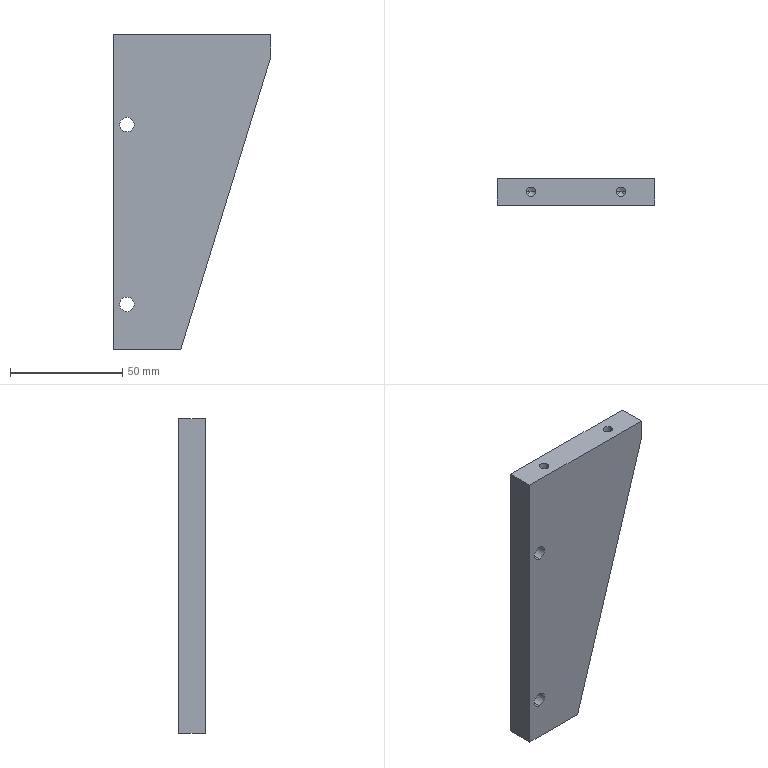Part | STEP file | PN_0033 | 1 solid | 19 faces | box 70 x 12 x 140 mm | volume 85204 mm3 | cylinder 8 | plane 7 | cone 4 | commonest cylinder face diameters 4.2 x4 6.5 x4
STEP:
#1=CARTESIAN_POINT('',(0.,0.,0.));
#2=DIRECTION('',(0.,0.,1.));
#3=DIRECTION('',(1.,0.,0.));
#4=AXIS2_PLACEMENT_3D('',#1,#2,#3);
#5=CARTESIAN_POINT('',(-17.9,6.,56.));
#6=VERTEX_POINT('',#5);
#7=CARTESIAN_POINT('',(-17.9,6.,70.));
#8=VERTEX_POINT('',#7);
#9=CARTESIAN_POINT('',(-17.9,6.,70.));
#10=DIRECTION('',(0.,0.,1.));
#11=VECTOR('',#10,1.);
#12=LINE('',#9,#11);
#13=CARTESIAN_POINT('',(-20.,6.,70.));
#14=DIRECTION('',(0.,0.,1.));
#15=DIRECTION('',(1.,0.,0.));
#16=AXIS2_PLACEMENT_3D('',#13,#14,#15);
#17=CYLINDRICAL_SURFACE('',#16,2.1);
#18=CARTESIAN_POINT('',(6.283,0.));
#19=DIRECTION('',(0.,1.));
#20=VECTOR('',#19,1.);
#21=LINE('',#18,#20);
#22=(GEOMETRIC_REPRESENTATION_CONTEXT(2)PARAMETRIC_REPRESENTATION_CONTEXT()REPRESENTATION_CONTEXT('',''));
#23=DEFINITIONAL_REPRESENTATION('',(#21),#22);
#24=PCURVE('',#17,#23);
#25=CARTESIAN_POINT('',(-20.,6.,70.));
#26=DIRECTION('',(0.,0.,1.));
#27=DIRECTION('',(1.,0.,0.));
#28=AXIS2_PLACEMENT_3D('',#25,#26,#27);
#29=CYLINDRICAL_SURFACE('',#28,2.1);
#30=CARTESIAN_POINT('',(0.,0.));
#31=DIRECTION('',(0.,1.));
#32=VECTOR('',#31,1.);
#33=LINE('',#30,#32);
#34=(GEOMETRIC_REPRESENTATION_CONTEXT(2)PARAMETRIC_REPRESENTATION_CONTEXT()REPRESENTATION_CONTEXT('',''));
#35=DEFINITIONAL_REPRESENTATION('',(#33),#34);
#36=PCURVE('',#29,#35);
#37=SURFACE_CURVE('',#12,(#24,#36),.PCURVE_S1.);
#38=EDGE_CURVE('',#6,#8,#37,.T.);
#39=ORIENTED_EDGE('',*,*,#38,.T.);
#40=CARTESIAN_POINT('',(-22.1,6.,70.));
#41=VERTEX_POINT('',#40);
#42=CARTESIAN_POINT('',(-20.,6.,70.));
#43=DIRECTION('',(0.,0.,1.));
#44=DIRECTION('',(1.,0.,0.));
#45=AXIS2_PLACEMENT_3D('',#42,#43,#44);
#46=CIRCLE('',#45,2.1);
#47=CARTESIAN_POINT('',(0.,0.));
#48=DIRECTION('',(1.,0.));
#49=VECTOR('',#48,1.);
#50=LINE('',#47,#49);
#51=(GEOMETRIC_REPRESENTATION_CONTEXT(2)PARAMETRIC_REPRESENTATION_CONTEXT()REPRESENTATION_CONTEXT('',''));
#52=DEFINITIONAL_REPRESENTATION('',(#50),#51);
#53=PCURVE('',#17,#52);
#54=CARTESIAN_POINT('',(-35.,12.,70.));
#55=DIRECTION('',(0.,0.,-1.));
#56=DIRECTION('',(-1.,0.,0.));
#57=AXIS2_PLACEMENT_3D('',#54,#55,#56);
#58=PLANE('',#57);
#59=CARTESIAN_POINT('',(-17.1,-6.));
#60=CARTESIAN_POINT('',(-17.1,-2.363));
#61=CARTESIAN_POINT('',(-13.95,-4.181));
#62=CARTESIAN_POINT('',(-10.8,-6.));
#63=CARTESIAN_POINT('',(-13.95,-7.819));
#64=CARTESIAN_POINT('',(-17.1,-9.637));
#65=CARTESIAN_POINT('',(-17.1,-6.));
#66=(BOUNDED_CURVE()B_SPLINE_CURVE(2,(#59,#60,#61,#62,#63,#64,#65),.UNSPECIFIED.,.T.,.F.)B_SPLINE_CURVE_WITH_KNOTS((1,2,2,2,2,1),(-2.094,0.,2.094,4.189,6.283,8.378),.UNSPECIFIED.)CURVE()GEOMETRIC_REPRESENTATION_ITEM()RATIONAL_B_SPLINE_CURVE((1.,0.5,1.,0.5,1.,0.5,1.))REPRESENTATION_ITEM(''));
#67=(GEOMETRIC_REPRESENTATION_CONTEXT(2)PARAMETRIC_REPRESENTATION_CONTEXT()REPRESENTATION_CONTEXT('',''));
#68=DEFINITIONAL_REPRESENTATION('',(#66),#67);
#69=PCURVE('',#58,#68);
#70=SURFACE_CURVE('',#46,(#53,#69),.PCURVE_S1.);
#71=EDGE_CURVE('',#41,#8,#70,.T.);
#72=ORIENTED_EDGE('',*,*,#71,.F.);
#73=CARTESIAN_POINT('',(-22.1,6.,56.));
#74=VERTEX_POINT('',#73);
#75=CARTESIAN_POINT('',(-22.1,6.,70.));
#76=DIRECTION('',(0.,0.,1.));
#77=VECTOR('',#76,1.);
#78=LINE('',#75,#77);
#79=CARTESIAN_POINT('',(3.142,0.));
#80=DIRECTION('',(0.,1.));
#81=VECTOR('',#80,1.);
#82=LINE('',#79,#81);
#83=(GEOMETRIC_REPRESENTATION_CONTEXT(2)PARAMETRIC_REPRESENTATION_CONTEXT()REPRESENTATION_CONTEXT('',''));
#84=DEFINITIONAL_REPRESENTATION('',(#82),#83);
#85=PCURVE('',#17,#84);
#86=CARTESIAN_POINT('',(3.142,0.));
#87=DIRECTION('',(0.,1.));
#88=VECTOR('',#87,1.);
#89=LINE('',#86,#88);
#90=(GEOMETRIC_REPRESENTATION_CONTEXT(2)PARAMETRIC_REPRESENTATION_CONTEXT()REPRESENTATION_CONTEXT('',''));
#91=DEFINITIONAL_REPRESENTATION('',(#89),#90);
#92=PCURVE('',#29,#91);
#93=SURFACE_CURVE('',#78,(#85,#92),.PCURVE_S1.);
#94=EDGE_CURVE('',#74,#41,#93,.T.);
#95=ORIENTED_EDGE('',*,*,#94,.F.);
#96=CARTESIAN_POINT('',(-20.,6.,56.));
#97=DIRECTION('',(0.,0.,1.));
#98=DIRECTION('',(1.,0.,0.));
#99=AXIS2_PLACEMENT_3D('',#96,#97,#98);
#100=CIRCLE('',#99,2.1);
#101=CARTESIAN_POINT('',(0.,-14.));
#102=DIRECTION('',(1.,0.));
#103=VECTOR('',#102,1.);
#104=LINE('',#101,#103);
#105=(GEOMETRIC_REPRESENTATION_CONTEXT(2)PARAMETRIC_REPRESENTATION_CONTEXT()REPRESENTATION_CONTEXT('',''));
#106=DEFINITIONAL_REPRESENTATION('',(#104),#105);
#107=PCURVE('',#17,#106);
#108=CARTESIAN_POINT('',(-20.,6.,56.));
#109=DIRECTION('',(0.,0.,1.));
#110=DIRECTION('',(1.,0.,0.));
#111=AXIS2_PLACEMENT_3D('',#108,#109,#110);
#112=CONICAL_SURFACE('',#111,2.1,1.03);
#113=CARTESIAN_POINT('',(0.,0.));
#114=DIRECTION('',(1.,0.));
#115=VECTOR('',#114,1.);
#116=LINE('',#113,#115);
#117=(GEOMETRIC_REPRESENTATION_CONTEXT(2)PARAMETRIC_REPRESENTATION_CONTEXT()REPRESENTATION_CONTEXT('',''));
#118=DEFINITIONAL_REPRESENTATION('',(#116),#117);
#119=PCURVE('',#112,#118);
#120=SURFACE_CURVE('',#100,(#107,#119),.PCURVE_S1.);
#121=EDGE_CURVE('',#74,#6,#120,.T.);
#122=ORIENTED_EDGE('',*,*,#121,.T.);
#123=EDGE_LOOP('',(#39,#72,#95,#122));
#124=FACE_BOUND('',#123,.F.);
#125=ADVANCED_FACE('',(#124),#17,.F.);
#126=ORIENTED_EDGE('',*,*,#121,.F.);
#127=CARTESIAN_POINT('',(-20.,6.,54.738));
#128=VERTEX_POINT('',#127);
#129=CARTESIAN_POINT('',(-22.1,6.,56.));
#130=DIRECTION('',(-0.8572,0.,0.515));
#131=VECTOR('',#130,1.);
#132=LINE('',#129,#131);
#133=CARTESIAN_POINT('',(3.142,0.));
#134=DIRECTION('',(0.,1.));
#135=VECTOR('',#134,1.);
#136=LINE('',#133,#135);
#137=(GEOMETRIC_REPRESENTATION_CONTEXT(2)PARAMETRIC_REPRESENTATION_CONTEXT()REPRESENTATION_CONTEXT('',''));
#138=DEFINITIONAL_REPRESENTATION('',(#136),#137);
#139=PCURVE('',#112,#138);
#140=CARTESIAN_POINT('',(-20.,6.,56.));
#141=DIRECTION('',(0.,0.,1.));
#142=DIRECTION('',(1.,0.,0.));
#143=AXIS2_PLACEMENT_3D('',#140,#141,#142);
#144=CONICAL_SURFACE('',#143,2.1,1.03);
#145=CARTESIAN_POINT('',(3.142,0.));
#146=DIRECTION('',(0.,1.));
#147=VECTOR('',#146,1.);
#148=LINE('',#145,#147);
#149=(GEOMETRIC_REPRESENTATION_CONTEXT(2)PARAMETRIC_REPRESENTATION_CONTEXT()REPRESENTATION_CONTEXT('',''));
#150=DEFINITIONAL_REPRESENTATION('',(#148),#149);
#151=PCURVE('',#144,#150);
#152=SURFACE_CURVE('',#132,(#139,#151),.PCURVE_S1.);
#153=EDGE_CURVE('',#128,#74,#152,.T.);
#154=ORIENTED_EDGE('',*,*,#153,.F.);
#155=CARTESIAN_POINT('',(-17.9,6.,56.));
#156=DIRECTION('',(0.8572,0.,0.515));
#157=VECTOR('',#156,1.);
#158=LINE('',#155,#157);
#159=CARTESIAN_POINT('',(6.283,0.));
#160=DIRECTION('',(0.,1.));
#161=VECTOR('',#160,1.);
#162=LINE('',#159,#161);
#163=(GEOMETRIC_REPRESENTATION_CONTEXT(2)PARAMETRIC_REPRESENTATION_CONTEXT()REPRESENTATION_CONTEXT('',''));
#164=DEFINITIONAL_REPRESENTATION('',(#162),#163);
#165=PCURVE('',#112,#164);
#166=CARTESIAN_POINT('',(0.,0.));
#167=DIRECTION('',(0.,1.));
#168=VECTOR('',#167,1.);
#169=LINE('',#166,#168);
#170=(GEOMETRIC_REPRESENTATION_CONTEXT(2)PARAMETRIC_REPRESENTATION_CONTEXT()REPRESENTATION_CONTEXT('',''));
#171=DEFINITIONAL_REPRESENTATION('',(#169),#170);
#172=PCURVE('',#144,#171);
#173=SURFACE_CURVE('',#158,(#165,#172),.PCURVE_S1.);
#174=EDGE_CURVE('',#128,#6,#173,.T.);
#175=ORIENTED_EDGE('',*,*,#174,.T.);
#176=EDGE_LOOP('',(#126,#154,#175));
#177=FACE_BOUND('',#176,.F.);
#178=ADVANCED_FACE('',(#177),#112,.F.);
#179=CARTESIAN_POINT('',(22.1,6.,56.));
#180=VERTEX_POINT('',#179);
#181=CARTESIAN_POINT('',(22.1,6.,70.));
#182=VERTEX_POINT('',#181);
#183=CARTESIAN_POINT('',(22.1,6.,70.));
#184=DIRECTION('',(0.,0.,1.));
#185=VECTOR('',#184,1.);
#186=LINE('',#183,#185);
#187=CARTESIAN_POINT('',(20.,6.,70.));
#188=DIRECTION('',(0.,0.,1.));
#189=DIRECTION('',(1.,0.,0.));
#190=AXIS2_PLACEMENT_3D('',#187,#188,#189);
#191=CYLINDRICAL_SURFACE('',#190,2.1);
#192=CARTESIAN_POINT('',(6.283,0.));
#193=DIRECTION('',(0.,1.));
#194=VECTOR('',#193,1.);
#195=LINE('',#192,#194);
#196=(GEOMETRIC_REPRESENTATION_CONTEXT(2)PARAMETRIC_REPRESENTATION_CONTEXT()REPRESENTATION_CONTEXT('',''));
#197=DEFINITIONAL_REPRESENTATION('',(#195),#196);
#198=PCURVE('',#191,#197);
#199=CARTESIAN_POINT('',(20.,6.,70.));
#200=DIRECTION('',(0.,0.,1.));
#201=DIRECTION('',(1.,0.,0.));
#202=AXIS2_PLACEMENT_3D('',#199,#200,#201);
#203=CYLINDRICAL_SURFACE('',#202,2.1);
#204=CARTESIAN_POINT('',(0.,0.));
#205=DIRECTION('',(0.,1.));
#206=VECTOR('',#205,1.);
#207=LINE('',#204,#206);
#208=(GEOMETRIC_REPRESENTATION_CONTEXT(2)PARAMETRIC_REPRESENTATION_CONTEXT()REPRESENTATION_CONTEXT('',''));
#209=DEFINITIONAL_REPRESENTATION('',(#207),#208);
#210=PCURVE('',#203,#209);
#211=SURFACE_CURVE('',#186,(#198,#210),.PCURVE_S1.);
#212=EDGE_CURVE('',#180,#182,#211,.T.);
#213=ORIENTED_EDGE('',*,*,#212,.T.);
#214=CARTESIAN_POINT('',(17.9,6.,70.));
#215=VERTEX_POINT('',#214);
#216=CARTESIAN_POINT('',(20.,6.,70.));
#217=DIRECTION('',(0.,0.,1.));
#218=DIRECTION('',(1.,0.,0.));
#219=AXIS2_PLACEMENT_3D('',#216,#217,#218);
#220=CIRCLE('',#219,2.1);
#221=CARTESIAN_POINT('',(0.,0.));
#222=DIRECTION('',(1.,0.));
#223=VECTOR('',#222,1.);
#224=LINE('',#221,#223);
#225=(GEOMETRIC_REPRESENTATION_CONTEXT(2)PARAMETRIC_REPRESENTATION_CONTEXT()REPRESENTATION_CONTEXT('',''));
#226=DEFINITIONAL_REPRESENTATION('',(#224),#225);
#227=PCURVE('',#191,#226);
#228=CARTESIAN_POINT('',(-57.1,-6.));
#229=CARTESIAN_POINT('',(-57.1,-2.363));
#230=CARTESIAN_POINT('',(-53.95,-4.181));
#231=CARTESIAN_POINT('',(-50.8,-6.));
#232=CARTESIAN_POINT('',(-53.95,-7.819));
#233=CARTESIAN_POINT('',(-57.1,-9.637));
#234=CARTESIAN_POINT('',(-57.1,-6.));
#235=(BOUNDED_CURVE()B_SPLINE_CURVE(2,(#228,#229,#230,#231,#232,#233,#234),.UNSPECIFIED.,.T.,.F.)B_SPLINE_CURVE_WITH_KNOTS((1,2,2,2,2,1),(-2.094,0.,2.094,4.189,6.283,8.378),.UNSPECIFIED.)CURVE()GEOMETRIC_REPRESENTATION_ITEM()RATIONAL_B_SPLINE_CURVE((1.,0.5,1.,0.5,1.,0.5,1.))REPRESENTATION_ITEM(''));
#236=(GEOMETRIC_REPRESENTATION_CONTEXT(2)PARAMETRIC_REPRESENTATION_CONTEXT()REPRESENTATION_CONTEXT('',''));
#237=DEFINITIONAL_REPRESENTATION('',(#235),#236);
#238=PCURVE('',#58,#237);
#239=SURFACE_CURVE('',#220,(#227,#238),.PCURVE_S1.);
#240=EDGE_CURVE('',#215,#182,#239,.T.);
#241=ORIENTED_EDGE('',*,*,#240,.F.);
#242=CARTESIAN_POINT('',(17.9,6.,56.));
#243=VERTEX_POINT('',#242);
#244=CARTESIAN_POINT('',(17.9,6.,70.));
#245=DIRECTION('',(0.,0.,1.));
#246=VECTOR('',#245,1.);
#247=LINE('',#244,#246);
#248=CARTESIAN_POINT('',(3.142,0.));
#249=DIRECTION('',(0.,1.));
#250=VECTOR('',#249,1.);
#251=LINE('',#248,#250);
#252=(GEOMETRIC_REPRESENTATION_CONTEXT(2)PARAMETRIC_REPRESENTATION_CONTEXT()REPRESENTATION_CONTEXT('',''));
#253=DEFINITIONAL_REPRESENTATION('',(#251),#252);
#254=PCURVE('',#191,#253);
#255=CARTESIAN_POINT('',(3.142,0.));
#256=DIRECTION('',(0.,1.));
#257=VECTOR('',#256,1.);
#258=LINE('',#255,#257);
#259=(GEOMETRIC_REPRESENTATION_CONTEXT(2)PARAMETRIC_REPRESENTATION_CONTEXT()REPRESENTATION_CONTEXT('',''));
#260=DEFINITIONAL_REPRESENTATION('',(#258),#259);
#261=PCURVE('',#203,#260);
#262=SURFACE_CURVE('',#247,(#254,#261),.PCURVE_S1.);
#263=EDGE_CURVE('',#243,#215,#262,.T.);
#264=ORIENTED_EDGE('',*,*,#263,.F.);
#265=CARTESIAN_POINT('',(20.,6.,56.));
#266=DIRECTION('',(0.,0.,1.));
#267=DIRECTION('',(1.,0.,0.));
#268=AXIS2_PLACEMENT_3D('',#265,#266,#267);
#269=CIRCLE('',#268,2.1);
#270=CARTESIAN_POINT('',(0.,-14.));
#271=DIRECTION('',(1.,0.));
#272=VECTOR('',#271,1.);
#273=LINE('',#270,#272);
#274=(GEOMETRIC_REPRESENTATION_CONTEXT(2)PARAMETRIC_REPRESENTATION_CONTEXT()REPRESENTATION_CONTEXT('',''));
#275=DEFINITIONAL_REPRESENTATION('',(#273),#274);
#276=PCURVE('',#191,#275);
#277=CARTESIAN_POINT('',(20.,6.,56.));
#278=DIRECTION('',(0.,0.,1.));
#279=DIRECTION('',(1.,0.,0.));
#280=AXIS2_PLACEMENT_3D('',#277,#278,#279);
#281=CONICAL_SURFACE('',#280,2.1,1.03);
#282=CARTESIAN_POINT('',(0.,0.));
#283=DIRECTION('',(1.,0.));
#284=VECTOR('',#283,1.);
#285=LINE('',#282,#284);
#286=(GEOMETRIC_REPRESENTATION_CONTEXT(2)PARAMETRIC_REPRESENTATION_CONTEXT()REPRESENTATION_CONTEXT('',''));
#287=DEFINITIONAL_REPRESENTATION('',(#285),#286);
#288=PCURVE('',#281,#287);
#289=SURFACE_CURVE('',#269,(#276,#288),.PCURVE_S1.);
#290=EDGE_CURVE('',#243,#180,#289,.T.);
#291=ORIENTED_EDGE('',*,*,#290,.T.);
#292=EDGE_LOOP('',(#213,#241,#264,#291));
#293=FACE_BOUND('',#292,.F.);
#294=ADVANCED_FACE('',(#293),#191,.F.);
#295=ORIENTED_EDGE('',*,*,#290,.F.);
#296=CARTESIAN_POINT('',(20.,6.,54.738));
#297=VERTEX_POINT('',#296);
#298=CARTESIAN_POINT('',(17.9,6.,56.));
#299=DIRECTION('',(-0.8572,0.,0.515));
#300=VECTOR('',#299,1.);
#301=LINE('',#298,#300);
#302=CARTESIAN_POINT('',(3.142,0.));
#303=DIRECTION('',(0.,1.));
#304=VECTOR('',#303,1.);
#305=LINE('',#302,#304);
#306=(GEOMETRIC_REPRESENTATION_CONTEXT(2)PARAMETRIC_REPRESENTATION_CONTEXT()REPRESENTATION_CONTEXT('',''));
#307=DEFINITIONAL_REPRESENTATION('',(#305),#306);
#308=PCURVE('',#281,#307);
#309=CARTESIAN_POINT('',(20.,6.,56.));
#310=DIRECTION('',(0.,0.,1.));
#311=DIRECTION('',(1.,0.,0.));
#312=AXIS2_PLACEMENT_3D('',#309,#310,#311);
#313=CONICAL_SURFACE('',#312,2.1,1.03);
#314=CARTESIAN_POINT('',(3.142,0.));
#315=DIRECTION('',(0.,1.));
#316=VECTOR('',#315,1.);
#317=LINE('',#314,#316);
#318=(GEOMETRIC_REPRESENTATION_CONTEXT(2)PARAMETRIC_REPRESENTATION_CONTEXT()REPRESENTATION_CONTEXT('',''));
#319=DEFINITIONAL_REPRESENTATION('',(#317),#318);
#320=PCURVE('',#313,#319);
#321=SURFACE_CURVE('',#301,(#308,#320),.PCURVE_S1.);
#322=EDGE_CURVE('',#297,#243,#321,.T.);
#323=ORIENTED_EDGE('',*,*,#322,.F.);
#324=CARTESIAN_POINT('',(22.1,6.,56.));
#325=DIRECTION('',(0.8572,0.,0.515));
#326=VECTOR('',#325,1.);
#327=LINE('',#324,#326);
#328=CARTESIAN_POINT('',(6.283,0.));
#329=DIRECTION('',(0.,1.));
#330=VECTOR('',#329,1.);
#331=LINE('',#328,#330);
#332=(GEOMETRIC_REPRESENTATION_CONTEXT(2)PARAMETRIC_REPRESENTATION_CONTEXT()REPRESENTATION_CONTEXT('',''));
#333=DEFINITIONAL_REPRESENTATION('',(#331),#332);
#334=PCURVE('',#281,#333);
#335=CARTESIAN_POINT('',(0.,0.));
#336=DIRECTION('',(0.,1.));
#337=VECTOR('',#336,1.);
#338=LINE('',#335,#337);
#339=(GEOMETRIC_REPRESENTATION_CONTEXT(2)PARAMETRIC_REPRESENTATION_CONTEXT()REPRESENTATION_CONTEXT('',''));
#340=DEFINITIONAL_REPRESENTATION('',(#338),#339);
#341=PCURVE('',#313,#340);
#342=SURFACE_CURVE('',#327,(#334,#341),.PCURVE_S1.);
#343=EDGE_CURVE('',#297,#180,#342,.T.);
#344=ORIENTED_EDGE('',*,*,#343,.T.);
#345=EDGE_LOOP('',(#295,#323,#344));
#346=FACE_BOUND('',#345,.F.);
#347=ADVANCED_FACE('',(#346),#281,.F.);
#348=CARTESIAN_POINT('',(-29.,12.,-53.25));
#349=VERTEX_POINT('',#348);
#350=CARTESIAN_POINT('',(-29.,0.,-53.25));
#351=VERTEX_POINT('',#350);
#352=CARTESIAN_POINT('',(-29.,0.,-53.25));
#353=DIRECTION('',(0.,-1.,0.));
#354=VECTOR('',#353,1.);
#355=LINE('',#352,#354);
#356=CARTESIAN_POINT('',(-29.,0.,-50.));
#357=DIRECTION('',(0.,-1.,0.));
#358=DIRECTION('',(0.,0.,-1.));
#359=AXIS2_PLACEMENT_3D('',#356,#357,#358);
#360=CYLINDRICAL_SURFACE('',#359,3.25);
#361=CARTESIAN_POINT('',(6.283,0.));
#362=DIRECTION('',(0.,1.));
#363=VECTOR('',#362,1.);
#364=LINE('',#361,#363);
#365=(GEOMETRIC_REPRESENTATION_CONTEXT(2)PARAMETRIC_REPRESENTATION_CONTEXT()REPRESENTATION_CONTEXT('',''));
#366=DEFINITIONAL_REPRESENTATION('',(#364),#365);
#367=PCURVE('',#360,#366);
#368=CARTESIAN_POINT('',(-29.,0.,-50.));
#369=DIRECTION('',(0.,-1.,0.));
#370=DIRECTION('',(0.,0.,-1.));
#371=AXIS2_PLACEMENT_3D('',#368,#369,#370);
#372=CYLINDRICAL_SURFACE('',#371,3.25);
#373=CARTESIAN_POINT('',(0.,0.));
#374=DIRECTION('',(0.,1.));
#375=VECTOR('',#374,1.);
#376=LINE('',#373,#375);
#377=(GEOMETRIC_REPRESENTATION_CONTEXT(2)PARAMETRIC_REPRESENTATION_CONTEXT()REPRESENTATION_CONTEXT('',''));
#378=DEFINITIONAL_REPRESENTATION('',(#376),#377);
#379=PCURVE('',#372,#378);
#380=SURFACE_CURVE('',#355,(#367,#379),.PCURVE_S1.);
#381=EDGE_CURVE('',#349,#351,#380,.T.);
#382=ORIENTED_EDGE('',*,*,#381,.T.);
#383=CARTESIAN_POINT('',(-29.,0.,-46.75));
#384=VERTEX_POINT('',#383);
#385=CARTESIAN_POINT('',(-29.,0.,-50.));
#386=DIRECTION('',(0.,-1.,0.));
#387=DIRECTION('',(0.,0.,-1.));
#388=AXIS2_PLACEMENT_3D('',#385,#386,#387);
#389=CIRCLE('',#388,3.25);
#390=CARTESIAN_POINT('',(0.,0.));
#391=DIRECTION('',(1.,0.));
#392=VECTOR('',#391,1.);
#393=LINE('',#390,#392);
#394=(GEOMETRIC_REPRESENTATION_CONTEXT(2)PARAMETRIC_REPRESENTATION_CONTEXT()REPRESENTATION_CONTEXT('',''));
#395=DEFINITIONAL_REPRESENTATION('',(#393),#394);
#396=PCURVE('',#360,#395);
#397=CARTESIAN_POINT('',(0.,0.,0.));
#398=DIRECTION('',(0.,-1.,0.));
#399=DIRECTION('',(0.,0.,-1.));
#400=AXIS2_PLACEMENT_3D('',#397,#398,#399);
#401=PLANE('',#400);
#402=CARTESIAN_POINT('',(50.,-29.));
#403=DIRECTION('',(1.,0.));
#404=AXIS2_PLACEMENT_2D('',#402,#403);
#405=CIRCLE('',#404,3.25);
#406=(GEOMETRIC_REPRESENTATION_CONTEXT(2)PARAMETRIC_REPRESENTATION_CONTEXT()REPRESENTATION_CONTEXT('',''));
#407=DEFINITIONAL_REPRESENTATION('',(#405),#406);
#408=PCURVE('',#401,#407);
#409=SURFACE_CURVE('',#389,(#396,#408),.PCURVE_S1.);
#410=EDGE_CURVE('',#384,#351,#409,.T.);
#411=ORIENTED_EDGE('',*,*,#410,.F.);
#412=CARTESIAN_POINT('',(-29.,12.,-46.75));
#413=VERTEX_POINT('',#412);
#414=CARTESIAN_POINT('',(-29.,0.,-46.75));
#415=DIRECTION('',(0.,-1.,0.));
#416=VECTOR('',#415,1.);
#417=LINE('',#414,#416);
#418=CARTESIAN_POINT('',(3.142,0.));
#419=DIRECTION('',(0.,1.));
#420=VECTOR('',#419,1.);
#421=LINE('',#418,#420);
#422=(GEOMETRIC_REPRESENTATION_CONTEXT(2)PARAMETRIC_REPRESENTATION_CONTEXT()REPRESENTATION_CONTEXT('',''));
#423=DEFINITIONAL_REPRESENTATION('',(#421),#422);
#424=PCURVE('',#360,#423);
#425=CARTESIAN_POINT('',(3.142,0.));
#426=DIRECTION('',(0.,1.));
#427=VECTOR('',#426,1.);
#428=LINE('',#425,#427);
#429=(GEOMETRIC_REPRESENTATION_CONTEXT(2)PARAMETRIC_REPRESENTATION_CONTEXT()REPRESENTATION_CONTEXT('',''));
#430=DEFINITIONAL_REPRESENTATION('',(#428),#429);
#431=PCURVE('',#372,#430);
#432=SURFACE_CURVE('',#417,(#424,#431),.PCURVE_S1.);
#433=EDGE_CURVE('',#413,#384,#432,.T.);
#434=ORIENTED_EDGE('',*,*,#433,.F.);
#435=CARTESIAN_POINT('',(-29.,12.,-50.));
#436=DIRECTION('',(0.,-1.,0.));
#437=DIRECTION('',(0.,0.,-1.));
#438=AXIS2_PLACEMENT_3D('',#435,#436,#437);
#439=CIRCLE('',#438,3.25);
#440=CARTESIAN_POINT('',(0.,-12.));
#441=DIRECTION('',(1.,0.));
#442=VECTOR('',#441,1.);
#443=LINE('',#440,#442);
#444=(GEOMETRIC_REPRESENTATION_CONTEXT(2)PARAMETRIC_REPRESENTATION_CONTEXT()REPRESENTATION_CONTEXT('',''));
#445=DEFINITIONAL_REPRESENTATION('',(#443),#444);
#446=PCURVE('',#360,#445);
#447=CARTESIAN_POINT('',(0.,12.,0.));
#448=DIRECTION('',(0.,-1.,0.));
#449=DIRECTION('',(0.,0.,-1.));
#450=AXIS2_PLACEMENT_3D('',#447,#448,#449);
#451=PLANE('',#450);
#452=CARTESIAN_POINT('',(50.,-29.));
#453=DIRECTION('',(1.,0.));
#454=AXIS2_PLACEMENT_2D('',#452,#453);
#455=CIRCLE('',#454,3.25);
#456=(GEOMETRIC_REPRESENTATION_CONTEXT(2)PARAMETRIC_REPRESENTATION_CONTEXT()REPRESENTATION_CONTEXT('',''));
#457=DEFINITIONAL_REPRESENTATION('',(#455),#456);
#458=PCURVE('',#451,#457);
#459=SURFACE_CURVE('',#439,(#446,#458),.PCURVE_S1.);
#460=EDGE_CURVE('',#413,#349,#459,.T.);
#461=ORIENTED_EDGE('',*,*,#460,.T.);
#462=EDGE_LOOP('',(#382,#411,#434,#461));
#463=FACE_BOUND('',#462,.F.);
#464=ADVANCED_FACE('',(#463),#360,.F.);
#465=CARTESIAN_POINT('',(-29.,12.,26.75));
#466=VERTEX_POINT('',#465);
#467=CARTESIAN_POINT('',(-29.,0.,26.75));
#468=VERTEX_POINT('',#467);
#469=CARTESIAN_POINT('',(-29.,0.,26.75));
#470=DIRECTION('',(0.,-1.,0.));
#471=VECTOR('',#470,1.);
#472=LINE('',#469,#471);
#473=CARTESIAN_POINT('',(-29.,0.,30.));
#474=DIRECTION('',(0.,-1.,0.));
#475=DIRECTION('',(0.,0.,-1.));
#476=AXIS2_PLACEMENT_3D('',#473,#474,#475);
#477=CYLINDRICAL_SURFACE('',#476,3.25);
#478=CARTESIAN_POINT('',(6.283,0.));
#479=DIRECTION('',(0.,1.));
#480=VECTOR('',#479,1.);
#481=LINE('',#478,#480);
#482=(GEOMETRIC_REPRESENTATION_CONTEXT(2)PARAMETRIC_REPRESENTATION_CONTEXT()REPRESENTATION_CONTEXT('',''));
#483=DEFINITIONAL_REPRESENTATION('',(#481),#482);
#484=PCURVE('',#477,#483);
#485=CARTESIAN_POINT('',(-29.,0.,30.));
#486=DIRECTION('',(0.,-1.,0.));
#487=DIRECTION('',(0.,0.,-1.));
#488=AXIS2_PLACEMENT_3D('',#485,#486,#487);
#489=CYLINDRICAL_SURFACE('',#488,3.25);
#490=CARTESIAN_POINT('',(0.,0.));
#491=DIRECTION('',(0.,1.));
#492=VECTOR('',#491,1.);
#493=LINE('',#490,#492);
#494=(GEOMETRIC_REPRESENTATION_CONTEXT(2)PARAMETRIC_REPRESENTATION_CONTEXT()REPRESENTATION_CONTEXT('',''));
#495=DEFINITIONAL_REPRESENTATION('',(#493),#494);
#496=PCURVE('',#489,#495);
#497=SURFACE_CURVE('',#472,(#484,#496),.PCURVE_S1.);
#498=EDGE_CURVE('',#466,#468,#497,.T.);
#499=ORIENTED_EDGE('',*,*,#498,.T.);
#500=CARTESIAN_POINT('',(-29.,0.,33.25));
#501=VERTEX_POINT('',#500);
#502=CARTESIAN_POINT('',(-29.,0.,30.));
#503=DIRECTION('',(0.,-1.,0.));
#504=DIRECTION('',(0.,0.,-1.));
#505=AXIS2_PLACEMENT_3D('',#502,#503,#504);
#506=CIRCLE('',#505,3.25);
#507=CARTESIAN_POINT('',(0.,0.));
#508=DIRECTION('',(1.,0.));
#509=VECTOR('',#508,1.);
#510=LINE('',#507,#509);
#511=(GEOMETRIC_REPRESENTATION_CONTEXT(2)PARAMETRIC_REPRESENTATION_CONTEXT()REPRESENTATION_CONTEXT('',''));
#512=DEFINITIONAL_REPRESENTATION('',(#510),#511);
#513=PCURVE('',#477,#512);
#514=CARTESIAN_POINT('',(-30.,-29.));
#515=DIRECTION('',(1.,0.));
#516=AXIS2_PLACEMENT_2D('',#514,#515);
#517=CIRCLE('',#516,3.25);
#518=(GEOMETRIC_REPRESENTATION_CONTEXT(2)PARAMETRIC_REPRESENTATION_CONTEXT()REPRESENTATION_CONTEXT('',''));
#519=DEFINITIONAL_REPRESENTATION('',(#517),#518);
#520=PCURVE('',#401,#519);
#521=SURFACE_CURVE('',#506,(#513,#520),.PCURVE_S1.);
#522=EDGE_CURVE('',#501,#468,#521,.T.);
#523=ORIENTED_EDGE('',*,*,#522,.F.);
#524=CARTESIAN_POINT('',(-29.,12.,33.25));
#525=VERTEX_POINT('',#524);
#526=CARTESIAN_POINT('',(-29.,0.,33.25));
#527=DIRECTION('',(0.,-1.,0.));
#528=VECTOR('',#527,1.);
#529=LINE('',#526,#528);
#530=CARTESIAN_POINT('',(3.142,0.));
#531=DIRECTION('',(0.,1.));
#532=VECTOR('',#531,1.);
#533=LINE('',#530,#532);
#534=(GEOMETRIC_REPRESENTATION_CONTEXT(2)PARAMETRIC_REPRESENTATION_CONTEXT()REPRESENTATION_CONTEXT('',''));
#535=DEFINITIONAL_REPRESENTATION('',(#533),#534);
#536=PCURVE('',#477,#535);
#537=CARTESIAN_POINT('',(3.142,0.));
#538=DIRECTION('',(0.,1.));
#539=VECTOR('',#538,1.);
#540=LINE('',#537,#539);
#541=(GEOMETRIC_REPRESENTATION_CONTEXT(2)PARAMETRIC_REPRESENTATION_CONTEXT()REPRESENTATION_CONTEXT('',''));
#542=DEFINITIONAL_REPRESENTATION('',(#540),#541);
#543=PCURVE('',#489,#542);
#544=SURFACE_CURVE('',#529,(#536,#543),.PCURVE_S1.);
#545=EDGE_CURVE('',#525,#501,#544,.T.);
#546=ORIENTED_EDGE('',*,*,#545,.F.);
#547=CARTESIAN_POINT('',(-29.,12.,30.));
#548=DIRECTION('',(0.,-1.,0.));
#549=DIRECTION('',(0.,0.,-1.));
#550=AXIS2_PLACEMENT_3D('',#547,#548,#549);
#551=CIRCLE('',#550,3.25);
#552=CARTESIAN_POINT('',(0.,-12.));
#553=DIRECTION('',(1.,0.));
#554=VECTOR('',#553,1.);
#555=LINE('',#552,#554);
#556=(GEOMETRIC_REPRESENTATION_CONTEXT(2)PARAMETRIC_REPRESENTATION_CONTEXT()REPRESENTATION_CONTEXT('',''));
#557=DEFINITIONAL_REPRESENTATION('',(#555),#556);
#558=PCURVE('',#477,#557);
#559=CARTESIAN_POINT('',(-30.,-29.));
#560=DIRECTION('',(1.,0.));
#561=AXIS2_PLACEMENT_2D('',#559,#560);
#562=CIRCLE('',#561,3.25);
#563=(GEOMETRIC_REPRESENTATION_CONTEXT(2)PARAMETRIC_REPRESENTATION_CONTEXT()REPRESENTATION_CONTEXT('',''));
#564=DEFINITIONAL_REPRESENTATION('',(#562),#563);
#565=PCURVE('',#451,#564);
#566=SURFACE_CURVE('',#551,(#558,#565),.PCURVE_S1.);
#567=EDGE_CURVE('',#525,#466,#566,.T.);
#568=ORIENTED_EDGE('',*,*,#567,.T.);
#569=EDGE_LOOP('',(#499,#523,#546,#568));
#570=FACE_BOUND('',#569,.F.);
#571=ADVANCED_FACE('',(#570),#477,.F.);
#572=CARTESIAN_POINT('',(35.,0.,70.));
#573=VERTEX_POINT('',#572);
#574=CARTESIAN_POINT('',(35.,0.,60.));
#575=VERTEX_POINT('',#574);
#576=CARTESIAN_POINT('',(35.,0.,70.));
#577=DIRECTION('',(0.,0.,-1.));
#578=VECTOR('',#577,1.);
#579=LINE('',#576,#578);
#580=CARTESIAN_POINT('',(35.,12.,70.));
#581=DIRECTION('',(-1.,0.,0.));
#582=DIRECTION('',(0.,0.,1.));
#583=AXIS2_PLACEMENT_3D('',#580,#581,#582);
#584=PLANE('',#583);
#585=CARTESIAN_POINT('',(0.,-12.));
#586=DIRECTION('',(-1.,0.));
#587=VECTOR('',#586,1.);
#588=LINE('',#585,#587);
#589=(GEOMETRIC_REPRESENTATION_CONTEXT(2)PARAMETRIC_REPRESENTATION_CONTEXT()REPRESENTATION_CONTEXT('',''));
#590=DEFINITIONAL_REPRESENTATION('',(#588),#589);
#591=PCURVE('',#584,#590);
#592=CARTESIAN_POINT('',(-70.,35.));
#593=DIRECTION('',(1.,0.));
#594=VECTOR('',#593,1.);
#595=LINE('',#592,#594);
#596=(GEOMETRIC_REPRESENTATION_CONTEXT(2)PARAMETRIC_REPRESENTATION_CONTEXT()REPRESENTATION_CONTEXT('',''));
#597=DEFINITIONAL_REPRESENTATION('',(#595),#596);
#598=PCURVE('',#401,#597);
#599=SURFACE_CURVE('',#579,(#591,#598),.PCURVE_S1.);
#600=EDGE_CURVE('',#573,#575,#599,.T.);
#601=ORIENTED_EDGE('',*,*,#600,.T.);
#602=CARTESIAN_POINT('',(35.,12.,60.));
#603=VERTEX_POINT('',#602);
#604=CARTESIAN_POINT('',(35.,-53.,60.));
#605=DIRECTION('',(0.,1.,0.));
#606=VECTOR('',#605,1.);
#607=LINE('',#604,#606);
#608=CARTESIAN_POINT('',(-10.,-65.));
#609=DIRECTION('',(0.,1.));
#610=VECTOR('',#609,1.);
#611=LINE('',#608,#610);
#612=(GEOMETRIC_REPRESENTATION_CONTEXT(2)PARAMETRIC_REPRESENTATION_CONTEXT()REPRESENTATION_CONTEXT('',''));
#613=DEFINITIONAL_REPRESENTATION('',(#611),#612);
#614=PCURVE('',#584,#613);
#615=CARTESIAN_POINT('',(-5.,-53.,-70.));
#616=DIRECTION('',(-0.9558,0.,0.2941));
#617=DIRECTION('',(0.2941,0.,0.9558));
#618=AXIS2_PLACEMENT_3D('',#615,#616,#617);
#619=PLANE('',#618);
#620=CARTESIAN_POINT('',(136.015,0.));
#621=DIRECTION('',(0.,1.));
#622=VECTOR('',#621,1.);
#623=LINE('',#620,#622);
#624=(GEOMETRIC_REPRESENTATION_CONTEXT(2)PARAMETRIC_REPRESENTATION_CONTEXT()REPRESENTATION_CONTEXT('',''));
#625=DEFINITIONAL_REPRESENTATION('',(#623),#624);
#626=PCURVE('',#619,#625);
#627=SURFACE_CURVE('',#607,(#614,#626),.PCURVE_S1.);
#628=EDGE_CURVE('',#575,#603,#627,.T.);
#629=ORIENTED_EDGE('',*,*,#628,.T.);
#630=CARTESIAN_POINT('',(35.,12.,70.));
#631=VERTEX_POINT('',#630);
#632=CARTESIAN_POINT('',(35.,12.,70.));
#633=DIRECTION('',(0.,0.,-1.));
#634=VECTOR('',#633,1.);
#635=LINE('',#632,#634);
#636=CARTESIAN_POINT('',(0.,0.));
#637=DIRECTION('',(-1.,0.));
#638=VECTOR('',#637,1.);
#639=LINE('',#636,#638);
#640=(GEOMETRIC_REPRESENTATION_CONTEXT(2)PARAMETRIC_REPRESENTATION_CONTEXT()REPRESENTATION_CONTEXT('',''));
#641=DEFINITIONAL_REPRESENTATION('',(#639),#640);
#642=PCURVE('',#584,#641);
#643=CARTESIAN_POINT('',(-70.,35.));
#644=DIRECTION('',(1.,0.));
#645=VECTOR('',#644,1.);
#646=LINE('',#643,#645);
#647=(GEOMETRIC_REPRESENTATION_CONTEXT(2)PARAMETRIC_REPRESENTATION_CONTEXT()REPRESENTATION_CONTEXT('',''));
#648=DEFINITIONAL_REPRESENTATION('',(#646),#647);
#649=PCURVE('',#451,#648);
#650=SURFACE_CURVE('',#635,(#642,#649),.PCURVE_S1.);
#651=EDGE_CURVE('',#631,#603,#650,.T.);
#652=ORIENTED_EDGE('',*,*,#651,.F.);
#653=CARTESIAN_POINT('',(35.,12.,70.));
#654=DIRECTION('',(0.,-1.,0.));
#655=VECTOR('',#654,1.);
#656=LINE('',#653,#655);
#657=CARTESIAN_POINT('',(0.,0.));
#658=DIRECTION('',(0.,-1.));
#659=VECTOR('',#658,1.);
#660=LINE('',#657,#659);
#661=(GEOMETRIC_REPRESENTATION_CONTEXT(2)PARAMETRIC_REPRESENTATION_CONTEXT()REPRESENTATION_CONTEXT('',''));
#662=DEFINITIONAL_REPRESENTATION('',(#660),#661);
#663=PCURVE('',#584,#662);
#664=CARTESIAN_POINT('',(-70.,0.));
#665=DIRECTION('',(0.,-1.));
#666=VECTOR('',#665,1.);
#667=LINE('',#664,#666);
#668=(GEOMETRIC_REPRESENTATION_CONTEXT(2)PARAMETRIC_REPRESENTATION_CONTEXT()REPRESENTATION_CONTEXT('',''));
#669=DEFINITIONAL_REPRESENTATION('',(#667),#668);
#670=PCURVE('',#58,#669);
#671=SURFACE_CURVE('',#656,(#663,#670),.PCURVE_S1.);
#672=EDGE_CURVE('',#631,#573,#671,.T.);
#673=ORIENTED_EDGE('',*,*,#672,.T.);
#674=EDGE_LOOP('',(#601,#629,#652,#673));
#675=FACE_BOUND('',#674,.T.);
#676=ADVANCED_FACE('',(#675),#584,.F.);
#677=CARTESIAN_POINT('',(-5.,12.,-70.));
#678=VERTEX_POINT('',#677);
#679=CARTESIAN_POINT('',(-35.,12.,-70.));
#680=VERTEX_POINT('',#679);
#681=CARTESIAN_POINT('',(-35.,12.,-70.));
#682=DIRECTION('',(-1.,0.,0.));
#683=VECTOR('',#682,1.);
#684=LINE('',#681,#683);
#685=CARTESIAN_POINT('',(-35.,12.,-70.));
#686=DIRECTION('',(0.,0.,1.));
#687=DIRECTION('',(1.,0.,0.));
#688=AXIS2_PLACEMENT_3D('',#685,#686,#687);
#689=PLANE('',#688);
#690=CARTESIAN_POINT('',(0.,0.));
#691=DIRECTION('',(-1.,0.));
#692=VECTOR('',#691,1.);
#693=LINE('',#690,#692);
#694=(GEOMETRIC_REPRESENTATION_CONTEXT(2)PARAMETRIC_REPRESENTATION_CONTEXT()REPRESENTATION_CONTEXT('',''));
#695=DEFINITIONAL_REPRESENTATION('',(#693),#694);
#696=PCURVE('',#689,#695);
#697=CARTESIAN_POINT('',(70.,-35.));
#698=DIRECTION('',(0.,-1.));
#699=VECTOR('',#698,1.);
#700=LINE('',#697,#699);
#701=(GEOMETRIC_REPRESENTATION_CONTEXT(2)PARAMETRIC_REPRESENTATION_CONTEXT()REPRESENTATION_CONTEXT('',''));
#702=DEFINITIONAL_REPRESENTATION('',(#700),#701);
#703=PCURVE('',#451,#702);
#704=SURFACE_CURVE('',#684,(#696,#703),.PCURVE_S1.);
#705=EDGE_CURVE('',#678,#680,#704,.T.);
#706=ORIENTED_EDGE('',*,*,#705,.F.);
#707=CARTESIAN_POINT('',(-5.,0.,-70.));
#708=VERTEX_POINT('',#707);
#709=CARTESIAN_POINT('',(-5.,-53.,-70.));
#710=DIRECTION('',(0.,1.,0.));
#711=VECTOR('',#710,1.);
#712=LINE('',#709,#711);
#713=CARTESIAN_POINT('',(30.,-65.));
#714=DIRECTION('',(0.,1.));
#715=VECTOR('',#714,1.);
#716=LINE('',#713,#715);
#717=(GEOMETRIC_REPRESENTATION_CONTEXT(2)PARAMETRIC_REPRESENTATION_CONTEXT()REPRESENTATION_CONTEXT('',''));
#718=DEFINITIONAL_REPRESENTATION('',(#716),#717);
#719=PCURVE('',#689,#718);
#720=CARTESIAN_POINT('',(0.,0.));
#721=DIRECTION('',(0.,1.));
#722=VECTOR('',#721,1.);
#723=LINE('',#720,#722);
#724=(GEOMETRIC_REPRESENTATION_CONTEXT(2)PARAMETRIC_REPRESENTATION_CONTEXT()REPRESENTATION_CONTEXT('',''));
#725=DEFINITIONAL_REPRESENTATION('',(#723),#724);
#726=PCURVE('',#619,#725);
#727=SURFACE_CURVE('',#712,(#719,#726),.PCURVE_S1.);
#728=EDGE_CURVE('',#708,#678,#727,.T.);
#729=ORIENTED_EDGE('',*,*,#728,.F.);
#730=CARTESIAN_POINT('',(-35.,0.,-70.));
#731=VERTEX_POINT('',#730);
#732=CARTESIAN_POINT('',(-35.,0.,-70.));
#733=DIRECTION('',(-1.,0.,0.));
#734=VECTOR('',#733,1.);
#735=LINE('',#732,#734);
#736=CARTESIAN_POINT('',(0.,-12.));
#737=DIRECTION('',(-1.,0.));
#738=VECTOR('',#737,1.);
#739=LINE('',#736,#738);
#740=(GEOMETRIC_REPRESENTATION_CONTEXT(2)PARAMETRIC_REPRESENTATION_CONTEXT()REPRESENTATION_CONTEXT('',''));
#741=DEFINITIONAL_REPRESENTATION('',(#739),#740);
#742=PCURVE('',#689,#741);
#743=CARTESIAN_POINT('',(70.,-35.));
#744=DIRECTION('',(0.,-1.));
#745=VECTOR('',#744,1.);
#746=LINE('',#743,#745);
#747=(GEOMETRIC_REPRESENTATION_CONTEXT(2)PARAMETRIC_REPRESENTATION_CONTEXT()REPRESENTATION_CONTEXT('',''));
#748=DEFINITIONAL_REPRESENTATION('',(#746),#747);
#749=PCURVE('',#401,#748);
#750=SURFACE_CURVE('',#735,(#742,#749),.PCURVE_S1.);
#751=EDGE_CURVE('',#708,#731,#750,.T.);
#752=ORIENTED_EDGE('',*,*,#751,.T.);
#753=CARTESIAN_POINT('',(-35.,12.,-70.));
#754=DIRECTION('',(0.,-1.,0.));
#755=VECTOR('',#754,1.);
#756=LINE('',#753,#755);
#757=CARTESIAN_POINT('',(0.,0.));
#758=DIRECTION('',(0.,-1.));
#759=VECTOR('',#758,1.);
#760=LINE('',#757,#759);
#761=(GEOMETRIC_REPRESENTATION_CONTEXT(2)PARAMETRIC_REPRESENTATION_CONTEXT()REPRESENTATION_CONTEXT('',''));
#762=DEFINITIONAL_REPRESENTATION('',(#760),#761);
#763=PCURVE('',#689,#762);
#764=CARTESIAN_POINT('',(-35.,12.,70.));
#765=DIRECTION('',(1.,0.,0.));
#766=DIRECTION('',(0.,0.,-1.));
#767=AXIS2_PLACEMENT_3D('',#764,#765,#766);
#768=PLANE('',#767);
#769=CARTESIAN_POINT('',(140.,0.));
#770=DIRECTION('',(0.,-1.));
#771=VECTOR('',#770,1.);
#772=LINE('',#769,#771);
#773=(GEOMETRIC_REPRESENTATION_CONTEXT(2)PARAMETRIC_REPRESENTATION_CONTEXT()REPRESENTATION_CONTEXT('',''));
#774=DEFINITIONAL_REPRESENTATION('',(#772),#773);
#775=PCURVE('',#768,#774);
#776=SURFACE_CURVE('',#756,(#763,#775),.PCURVE_S1.);
#777=EDGE_CURVE('',#680,#731,#776,.T.);
#778=ORIENTED_EDGE('',*,*,#777,.F.);
#779=EDGE_LOOP('',(#706,#729,#752,#778));
#780=FACE_BOUND('',#779,.T.);
#781=ADVANCED_FACE('',(#780),#689,.F.);
#782=CARTESIAN_POINT('',(-35.,0.,70.));
#783=VERTEX_POINT('',#782);
#784=CARTESIAN_POINT('',(-35.,0.,70.));
#785=DIRECTION('',(0.,0.,1.));
#786=VECTOR('',#785,1.);
#787=LINE('',#784,#786);
#788=CARTESIAN_POINT('',(0.,-12.));
#789=DIRECTION('',(-1.,0.));
#790=VECTOR('',#789,1.);
#791=LINE('',#788,#790);
#792=(GEOMETRIC_REPRESENTATION_CONTEXT(2)PARAMETRIC_REPRESENTATION_CONTEXT()REPRESENTATION_CONTEXT('',''));
#793=DEFINITIONAL_REPRESENTATION('',(#791),#792);
#794=PCURVE('',#768,#793);
#795=CARTESIAN_POINT('',(-70.,-35.));
#796=DIRECTION('',(-1.,0.));
#797=VECTOR('',#796,1.);
#798=LINE('',#795,#797);
#799=(GEOMETRIC_REPRESENTATION_CONTEXT(2)PARAMETRIC_REPRESENTATION_CONTEXT()REPRESENTATION_CONTEXT('',''));
#800=DEFINITIONAL_REPRESENTATION('',(#798),#799);
#801=PCURVE('',#401,#800);
#802=SURFACE_CURVE('',#787,(#794,#801),.PCURVE_S1.);
#803=EDGE_CURVE('',#731,#783,#802,.T.);
#804=ORIENTED_EDGE('',*,*,#803,.T.);
#805=CARTESIAN_POINT('',(-35.,12.,70.));
#806=VERTEX_POINT('',#805);
#807=CARTESIAN_POINT('',(-35.,12.,70.));
#808=DIRECTION('',(0.,-1.,0.));
#809=VECTOR('',#808,1.);
#810=LINE('',#807,#809);
#811=CARTESIAN_POINT('',(0.,0.));
#812=DIRECTION('',(0.,-1.));
#813=VECTOR('',#812,1.);
#814=LINE('',#811,#813);
#815=(GEOMETRIC_REPRESENTATION_CONTEXT(2)PARAMETRIC_REPRESENTATION_CONTEXT()REPRESENTATION_CONTEXT('',''));
#816=DEFINITIONAL_REPRESENTATION('',(#814),#815);
#817=PCURVE('',#768,#816);
#818=CARTESIAN_POINT('',(0.,0.));
#819=DIRECTION('',(0.,-1.));
#820=VECTOR('',#819,1.);
#821=LINE('',#818,#820);
#822=(GEOMETRIC_REPRESENTATION_CONTEXT(2)PARAMETRIC_REPRESENTATION_CONTEXT()REPRESENTATION_CONTEXT('',''));
#823=DEFINITIONAL_REPRESENTATION('',(#821),#822);
#824=PCURVE('',#58,#823);
#825=SURFACE_CURVE('',#810,(#817,#824),.PCURVE_S1.);
#826=EDGE_CURVE('',#806,#783,#825,.T.);
#827=ORIENTED_EDGE('',*,*,#826,.F.);
#828=CARTESIAN_POINT('',(-35.,12.,70.));
#829=DIRECTION('',(0.,0.,1.));
#830=VECTOR('',#829,1.);
#831=LINE('',#828,#830);
#832=CARTESIAN_POINT('',(0.,0.));
#833=DIRECTION('',(-1.,0.));
#834=VECTOR('',#833,1.);
#835=LINE('',#832,#834);
#836=(GEOMETRIC_REPRESENTATION_CONTEXT(2)PARAMETRIC_REPRESENTATION_CONTEXT()REPRESENTATION_CONTEXT('',''));
#837=DEFINITIONAL_REPRESENTATION('',(#835),#836);
#838=PCURVE('',#768,#837);
#839=CARTESIAN_POINT('',(-70.,-35.));
#840=DIRECTION('',(-1.,0.));
#841=VECTOR('',#840,1.);
#842=LINE('',#839,#841);
#843=(GEOMETRIC_REPRESENTATION_CONTEXT(2)PARAMETRIC_REPRESENTATION_CONTEXT()REPRESENTATION_CONTEXT('',''));
#844=DEFINITIONAL_REPRESENTATION('',(#842),#843);
#845=PCURVE('',#451,#844);
#846=SURFACE_CURVE('',#831,(#838,#845),.PCURVE_S1.);
#847=EDGE_CURVE('',#680,#806,#846,.T.);
#848=ORIENTED_EDGE('',*,*,#847,.F.);
#849=ORIENTED_EDGE('',*,*,#777,.T.);
#850=EDGE_LOOP('',(#804,#827,#848,#849));
#851=FACE_BOUND('',#850,.T.);
#852=ADVANCED_FACE('',(#851),#768,.F.);
#853=CARTESIAN_POINT('',(-20.,6.,70.));
#854=DIRECTION('',(0.,0.,1.));
#855=DIRECTION('',(1.,0.,0.));
#856=AXIS2_PLACEMENT_3D('',#853,#854,#855);
#857=CIRCLE('',#856,2.1);
#858=CARTESIAN_POINT('',(-17.1,-6.));
#859=CARTESIAN_POINT('',(-17.1,-2.363));
#860=CARTESIAN_POINT('',(-13.95,-4.181));
#861=CARTESIAN_POINT('',(-10.8,-6.));
#862=CARTESIAN_POINT('',(-13.95,-7.819));
#863=CARTESIAN_POINT('',(-17.1,-9.637));
#864=CARTESIAN_POINT('',(-17.1,-6.));
#865=(BOUNDED_CURVE()B_SPLINE_CURVE(2,(#858,#859,#860,#861,#862,#863,#864),.UNSPECIFIED.,.T.,.F.)B_SPLINE_CURVE_WITH_KNOTS((1,2,2,2,2,1),(-2.094,0.,2.094,4.189,6.283,8.378),.UNSPECIFIED.)CURVE()GEOMETRIC_REPRESENTATION_ITEM()RATIONAL_B_SPLINE_CURVE((1.,0.5,1.,0.5,1.,0.5,1.))REPRESENTATION_ITEM(''));
#866=(GEOMETRIC_REPRESENTATION_CONTEXT(2)PARAMETRIC_REPRESENTATION_CONTEXT()REPRESENTATION_CONTEXT('',''));
#867=DEFINITIONAL_REPRESENTATION('',(#865),#866);
#868=PCURVE('',#58,#867);
#869=CARTESIAN_POINT('',(0.,0.));
#870=DIRECTION('',(1.,0.));
#871=VECTOR('',#870,1.);
#872=LINE('',#869,#871);
#873=(GEOMETRIC_REPRESENTATION_CONTEXT(2)PARAMETRIC_REPRESENTATION_CONTEXT()REPRESENTATION_CONTEXT('',''));
#874=DEFINITIONAL_REPRESENTATION('',(#872),#873);
#875=PCURVE('',#29,#874);
#876=SURFACE_CURVE('',#857,(#868,#875),.PCURVE_S1.);
#877=EDGE_CURVE('',#8,#41,#876,.T.);
#878=ORIENTED_EDGE('',*,*,#877,.F.);
#879=ORIENTED_EDGE('',*,*,#71,.F.);
#880=EDGE_LOOP('',(#878,#879));
#881=FACE_BOUND('',#880,.T.);
#882=CARTESIAN_POINT('',(20.,6.,70.));
#883=DIRECTION('',(0.,0.,1.));
#884=DIRECTION('',(1.,0.,0.));
#885=AXIS2_PLACEMENT_3D('',#882,#883,#884);
#886=CIRCLE('',#885,2.1);
#887=CARTESIAN_POINT('',(-57.1,-6.));
#888=CARTESIAN_POINT('',(-57.1,-2.363));
#889=CARTESIAN_POINT('',(-53.95,-4.181));
#890=CARTESIAN_POINT('',(-50.8,-6.));
#891=CARTESIAN_POINT('',(-53.95,-7.819));
#892=CARTESIAN_POINT('',(-57.1,-9.637));
#893=CARTESIAN_POINT('',(-57.1,-6.));
#894=(BOUNDED_CURVE()B_SPLINE_CURVE(2,(#887,#888,#889,#890,#891,#892,#893),.UNSPECIFIED.,.T.,.F.)B_SPLINE_CURVE_WITH_KNOTS((1,2,2,2,2,1),(-2.094,0.,2.094,4.189,6.283,8.378),.UNSPECIFIED.)CURVE()GEOMETRIC_REPRESENTATION_ITEM()RATIONAL_B_SPLINE_CURVE((1.,0.5,1.,0.5,1.,0.5,1.))REPRESENTATION_ITEM(''));
#895=(GEOMETRIC_REPRESENTATION_CONTEXT(2)PARAMETRIC_REPRESENTATION_CONTEXT()REPRESENTATION_CONTEXT('',''));
#896=DEFINITIONAL_REPRESENTATION('',(#894),#895);
#897=PCURVE('',#58,#896);
#898=CARTESIAN_POINT('',(0.,0.));
#899=DIRECTION('',(1.,0.));
#900=VECTOR('',#899,1.);
#901=LINE('',#898,#900);
#902=(GEOMETRIC_REPRESENTATION_CONTEXT(2)PARAMETRIC_REPRESENTATION_CONTEXT()REPRESENTATION_CONTEXT('',''));
#903=DEFINITIONAL_REPRESENTATION('',(#901),#902);
#904=PCURVE('',#203,#903);
#905=SURFACE_CURVE('',#886,(#897,#904),.PCURVE_S1.);
#906=EDGE_CURVE('',#182,#215,#905,.T.);
#907=ORIENTED_EDGE('',*,*,#906,.F.);
#908=ORIENTED_EDGE('',*,*,#240,.F.);
#909=EDGE_LOOP('',(#907,#908));
#910=FACE_BOUND('',#909,.T.);
#911=CARTESIAN_POINT('',(-35.,0.,70.));
#912=DIRECTION('',(1.,0.,0.));
#913=VECTOR('',#912,1.);
#914=LINE('',#911,#913);
#915=CARTESIAN_POINT('',(0.,-12.));
#916=DIRECTION('',(-1.,0.));
#917=VECTOR('',#916,1.);
#918=LINE('',#915,#917);
#919=(GEOMETRIC_REPRESENTATION_CONTEXT(2)PARAMETRIC_REPRESENTATION_CONTEXT()REPRESENTATION_CONTEXT('',''));
#920=DEFINITIONAL_REPRESENTATION('',(#918),#919);
#921=PCURVE('',#58,#920);
#922=CARTESIAN_POINT('',(-70.,-35.));
#923=DIRECTION('',(0.,1.));
#924=VECTOR('',#923,1.);
#925=LINE('',#922,#924);
#926=(GEOMETRIC_REPRESENTATION_CONTEXT(2)PARAMETRIC_REPRESENTATION_CONTEXT()REPRESENTATION_CONTEXT('',''));
#927=DEFINITIONAL_REPRESENTATION('',(#925),#926);
#928=PCURVE('',#401,#927);
#929=SURFACE_CURVE('',#914,(#921,#928),.PCURVE_S1.);
#930=EDGE_CURVE('',#783,#573,#929,.T.);
#931=ORIENTED_EDGE('',*,*,#930,.T.);
#932=ORIENTED_EDGE('',*,*,#672,.F.);
#933=CARTESIAN_POINT('',(-35.,12.,70.));
#934=DIRECTION('',(1.,0.,0.));
#935=VECTOR('',#934,1.);
#936=LINE('',#933,#935);
#937=CARTESIAN_POINT('',(0.,0.));
#938=DIRECTION('',(-1.,0.));
#939=VECTOR('',#938,1.);
#940=LINE('',#937,#939);
#941=(GEOMETRIC_REPRESENTATION_CONTEXT(2)PARAMETRIC_REPRESENTATION_CONTEXT()REPRESENTATION_CONTEXT('',''));
#942=DEFINITIONAL_REPRESENTATION('',(#940),#941);
#943=PCURVE('',#58,#942);
#944=CARTESIAN_POINT('',(-70.,-35.));
#945=DIRECTION('',(0.,1.));
#946=VECTOR('',#945,1.);
#947=LINE('',#944,#946);
#948=(GEOMETRIC_REPRESENTATION_CONTEXT(2)PARAMETRIC_REPRESENTATION_CONTEXT()REPRESENTATION_CONTEXT('',''));
#949=DEFINITIONAL_REPRESENTATION('',(#947),#948);
#950=PCURVE('',#451,#949);
#951=SURFACE_CURVE('',#936,(#943,#950),.PCURVE_S1.);
#952=EDGE_CURVE('',#806,#631,#951,.T.);
#953=ORIENTED_EDGE('',*,*,#952,.F.);
#954=ORIENTED_EDGE('',*,*,#826,.T.);
#955=EDGE_LOOP('',(#931,#932,#953,#954));
#956=FACE_BOUND('',#955,.T.);
#957=ADVANCED_FACE('',(#881,#910,#956),#58,.F.);
#958=CARTESIAN_POINT('',(-29.,12.,-50.));
#959=DIRECTION('',(0.,-1.,0.));
#960=DIRECTION('',(0.,0.,-1.));
#961=AXIS2_PLACEMENT_3D('',#958,#959,#960);
#962=CIRCLE('',#961,3.25);
#963=CARTESIAN_POINT('',(50.,-29.));
#964=DIRECTION('',(1.,0.));
#965=AXIS2_PLACEMENT_2D('',#963,#964);
#966=CIRCLE('',#965,3.25);
#967=(GEOMETRIC_REPRESENTATION_CONTEXT(2)PARAMETRIC_REPRESENTATION_CONTEXT()REPRESENTATION_CONTEXT('',''));
#968=DEFINITIONAL_REPRESENTATION('',(#966),#967);
#969=PCURVE('',#451,#968);
#970=CARTESIAN_POINT('',(0.,-12.));
#971=DIRECTION('',(1.,0.));
#972=VECTOR('',#971,1.);
#973=LINE('',#970,#972);
#974=(GEOMETRIC_REPRESENTATION_CONTEXT(2)PARAMETRIC_REPRESENTATION_CONTEXT()REPRESENTATION_CONTEXT('',''));
#975=DEFINITIONAL_REPRESENTATION('',(#973),#974);
#976=PCURVE('',#372,#975);
#977=SURFACE_CURVE('',#962,(#969,#976),.PCURVE_S1.);
#978=EDGE_CURVE('',#349,#413,#977,.T.);
#979=ORIENTED_EDGE('',*,*,#978,.T.);
#980=ORIENTED_EDGE('',*,*,#460,.T.);
#981=EDGE_LOOP('',(#979,#980));
#982=FACE_BOUND('',#981,.T.);
#983=CARTESIAN_POINT('',(-29.,12.,30.));
#984=DIRECTION('',(0.,-1.,0.));
#985=DIRECTION('',(0.,0.,-1.));
#986=AXIS2_PLACEMENT_3D('',#983,#984,#985);
#987=CIRCLE('',#986,3.25);
#988=CARTESIAN_POINT('',(-30.,-29.));
#989=DIRECTION('',(1.,0.));
#990=AXIS2_PLACEMENT_2D('',#988,#989);
#991=CIRCLE('',#990,3.25);
#992=(GEOMETRIC_REPRESENTATION_CONTEXT(2)PARAMETRIC_REPRESENTATION_CONTEXT()REPRESENTATION_CONTEXT('',''));
#993=DEFINITIONAL_REPRESENTATION('',(#991),#992);
#994=PCURVE('',#451,#993);
#995=CARTESIAN_POINT('',(0.,-12.));
#996=DIRECTION('',(1.,0.));
#997=VECTOR('',#996,1.);
#998=LINE('',#995,#997);
#999=(GEOMETRIC_REPRESENTATION_CONTEXT(2)PARAMETRIC_REPRESENTATION_CONTEXT()REPRESENTATION_CONTEXT('',''));
#1000=DEFINITIONAL_REPRESENTATION('',(#998),#999);
#1001=PCURVE('',#489,#1000);
#1002=SURFACE_CURVE('',#987,(#994,#1001),.PCURVE_S1.);
#1003=EDGE_CURVE('',#466,#525,#1002,.T.);
#1004=ORIENTED_EDGE('',*,*,#1003,.T.);
#1005=ORIENTED_EDGE('',*,*,#567,.T.);
#1006=EDGE_LOOP('',(#1004,#1005));
#1007=FACE_BOUND('',#1006,.T.);
#1008=ORIENTED_EDGE('',*,*,#651,.T.);
#1009=CARTESIAN_POINT('',(-5.,12.,-70.));
#1010=DIRECTION('',(0.2941,0.,0.9558));
#1011=VECTOR('',#1010,1.);
#1012=LINE('',#1009,#1011);
#1013=CARTESIAN_POINT('',(70.,-5.));
#1014=DIRECTION('',(-0.9558,0.2941));
#1015=VECTOR('',#1014,1.);
#1016=LINE('',#1013,#1015);
#1017=(GEOMETRIC_REPRESENTATION_CONTEXT(2)PARAMETRIC_REPRESENTATION_CONTEXT()REPRESENTATION_CONTEXT('',''));
#1018=DEFINITIONAL_REPRESENTATION('',(#1016),#1017);
#1019=PCURVE('',#451,#1018);
#1020=CARTESIAN_POINT('',(0.,65.));
#1021=DIRECTION('',(1.,0.));
#1022=VECTOR('',#1021,1.);
#1023=LINE('',#1020,#1022);
#1024=(GEOMETRIC_REPRESENTATION_CONTEXT(2)PARAMETRIC_REPRESENTATION_CONTEXT()REPRESENTATION_CONTEXT('',''));
#1025=DEFINITIONAL_REPRESENTATION('',(#1023),#1024);
#1026=PCURVE('',#619,#1025);
#1027=SURFACE_CURVE('',#1012,(#1019,#1026),.PCURVE_S1.);
#1028=EDGE_CURVE('',#678,#603,#1027,.T.);
#1029=ORIENTED_EDGE('',*,*,#1028,.F.);
#1030=ORIENTED_EDGE('',*,*,#705,.T.);
#1031=ORIENTED_EDGE('',*,*,#847,.T.);
#1032=ORIENTED_EDGE('',*,*,#952,.T.);
#1033=EDGE_LOOP('',(#1008,#1029,#1030,#1031,#1032));
#1034=FACE_BOUND('',#1033,.T.);
#1035=ADVANCED_FACE('',(#982,#1007,#1034),#451,.F.);
#1036=CARTESIAN_POINT('',(-29.,0.,-50.));
#1037=DIRECTION('',(0.,-1.,0.));
#1038=DIRECTION('',(0.,0.,-1.));
#1039=AXIS2_PLACEMENT_3D('',#1036,#1037,#1038);
#1040=CIRCLE('',#1039,3.25);
#1041=CARTESIAN_POINT('',(50.,-29.));
#1042=DIRECTION('',(1.,0.));
#1043=AXIS2_PLACEMENT_2D('',#1041,#1042);
#1044=CIRCLE('',#1043,3.25);
#1045=(GEOMETRIC_REPRESENTATION_CONTEXT(2)PARAMETRIC_REPRESENTATION_CONTEXT()REPRESENTATION_CONTEXT('',''));
#1046=DEFINITIONAL_REPRESENTATION('',(#1044),#1045);
#1047=PCURVE('',#401,#1046);
#1048=CARTESIAN_POINT('',(0.,0.));
#1049=DIRECTION('',(1.,0.));
#1050=VECTOR('',#1049,1.);
#1051=LINE('',#1048,#1050);
#1052=(GEOMETRIC_REPRESENTATION_CONTEXT(2)PARAMETRIC_REPRESENTATION_CONTEXT()REPRESENTATION_CONTEXT('',''));
#1053=DEFINITIONAL_REPRESENTATION('',(#1051),#1052);
#1054=PCURVE('',#372,#1053);
#1055=SURFACE_CURVE('',#1040,(#1047,#1054),.PCURVE_S1.);
#1056=EDGE_CURVE('',#351,#384,#1055,.T.);
#1057=ORIENTED_EDGE('',*,*,#1056,.F.);
#1058=ORIENTED_EDGE('',*,*,#410,.F.);
#1059=EDGE_LOOP('',(#1057,#1058));
#1060=FACE_BOUND('',#1059,.T.);
#1061=CARTESIAN_POINT('',(-29.,0.,30.));
#1062=DIRECTION('',(0.,-1.,0.));
#1063=DIRECTION('',(0.,0.,-1.));
#1064=AXIS2_PLACEMENT_3D('',#1061,#1062,#1063);
#1065=CIRCLE('',#1064,3.25);
#1066=CARTESIAN_POINT('',(-30.,-29.));
#1067=DIRECTION('',(1.,0.));
#1068=AXIS2_PLACEMENT_2D('',#1066,#1067);
#1069=CIRCLE('',#1068,3.25);
#1070=(GEOMETRIC_REPRESENTATION_CONTEXT(2)PARAMETRIC_REPRESENTATION_CONTEXT()REPRESENTATION_CONTEXT('',''));
#1071=DEFINITIONAL_REPRESENTATION('',(#1069),#1070);
#1072=PCURVE('',#401,#1071);
#1073=CARTESIAN_POINT('',(0.,0.));
#1074=DIRECTION('',(1.,0.));
#1075=VECTOR('',#1074,1.);
#1076=LINE('',#1073,#1075);
#1077=(GEOMETRIC_REPRESENTATION_CONTEXT(2)PARAMETRIC_REPRESENTATION_CONTEXT()REPRESENTATION_CONTEXT('',''));
#1078=DEFINITIONAL_REPRESENTATION('',(#1076),#1077);
#1079=PCURVE('',#489,#1078);
#1080=SURFACE_CURVE('',#1065,(#1072,#1079),.PCURVE_S1.);
#1081=EDGE_CURVE('',#468,#501,#1080,.T.);
#1082=ORIENTED_EDGE('',*,*,#1081,.F.);
#1083=ORIENTED_EDGE('',*,*,#522,.F.);
#1084=EDGE_LOOP('',(#1082,#1083));
#1085=FACE_BOUND('',#1084,.T.);
#1086=CARTESIAN_POINT('',(15.108,0.,-4.649));
#1087=DIRECTION('',(-0.2941,0.,-0.9558));
#1088=VECTOR('',#1087,1.);
#1089=LINE('',#1086,#1088);
#1090=CARTESIAN_POINT('',(4.649,15.108));
#1091=DIRECTION('',(0.9558,-0.2941));
#1092=VECTOR('',#1091,1.);
#1093=LINE('',#1090,#1092);
#1094=(GEOMETRIC_REPRESENTATION_CONTEXT(2)PARAMETRIC_REPRESENTATION_CONTEXT()REPRESENTATION_CONTEXT('',''));
#1095=DEFINITIONAL_REPRESENTATION('',(#1093),#1094);
#1096=PCURVE('',#401,#1095);
#1097=CARTESIAN_POINT('',(68.375,53.));
#1098=DIRECTION('',(-1.,0.));
#1099=VECTOR('',#1098,1.);
#1100=LINE('',#1097,#1099);
#1101=(GEOMETRIC_REPRESENTATION_CONTEXT(2)PARAMETRIC_REPRESENTATION_CONTEXT()REPRESENTATION_CONTEXT('',''));
#1102=DEFINITIONAL_REPRESENTATION('',(#1100),#1101);
#1103=PCURVE('',#619,#1102);
#1104=SURFACE_CURVE('',#1089,(#1096,#1103),.PCURVE_S1.);
#1105=EDGE_CURVE('',#575,#708,#1104,.T.);
#1106=ORIENTED_EDGE('',*,*,#1105,.F.);
#1107=ORIENTED_EDGE('',*,*,#600,.F.);
#1108=ORIENTED_EDGE('',*,*,#930,.F.);
#1109=ORIENTED_EDGE('',*,*,#803,.F.);
#1110=ORIENTED_EDGE('',*,*,#751,.F.);
#1111=EDGE_LOOP('',(#1106,#1107,#1108,#1109,#1110));
#1112=FACE_BOUND('',#1111,.T.);
#1113=ADVANCED_FACE('',(#1060,#1085,#1112),#401,.T.);
#1114=ORIENTED_EDGE('',*,*,#1105,.T.);
#1115=ORIENTED_EDGE('',*,*,#728,.T.);
#1116=ORIENTED_EDGE('',*,*,#1028,.T.);
#1117=ORIENTED_EDGE('',*,*,#628,.F.);
#1118=EDGE_LOOP('',(#1114,#1115,#1116,#1117));
#1119=FACE_BOUND('',#1118,.T.);
#1120=ADVANCED_FACE('',(#1119),#619,.F.);
#1121=ORIENTED_EDGE('',*,*,#1081,.F.);
#1122=ORIENTED_EDGE('',*,*,#498,.F.);
#1123=ORIENTED_EDGE('',*,*,#1003,.T.);
#1124=ORIENTED_EDGE('',*,*,#545,.T.);
#1125=EDGE_LOOP('',(#1121,#1122,#1123,#1124));
#1126=FACE_BOUND('',#1125,.F.);
#1127=ADVANCED_FACE('',(#1126),#489,.F.);
#1128=ORIENTED_EDGE('',*,*,#1056,.F.);
#1129=ORIENTED_EDGE('',*,*,#381,.F.);
#1130=ORIENTED_EDGE('',*,*,#978,.T.);
#1131=ORIENTED_EDGE('',*,*,#433,.T.);
#1132=EDGE_LOOP('',(#1128,#1129,#1130,#1131));
#1133=FACE_BOUND('',#1132,.F.);
#1134=ADVANCED_FACE('',(#1133),#372,.F.);
#1135=CARTESIAN_POINT('',(20.,6.,56.));
#1136=DIRECTION('',(0.,0.,1.));
#1137=DIRECTION('',(1.,0.,0.));
#1138=AXIS2_PLACEMENT_3D('',#1135,#1136,#1137);
#1139=CIRCLE('',#1138,2.1);
#1140=CARTESIAN_POINT('',(0.,0.));
#1141=DIRECTION('',(1.,0.));
#1142=VECTOR('',#1141,1.);
#1143=LINE('',#1140,#1142);
#1144=(GEOMETRIC_REPRESENTATION_CONTEXT(2)PARAMETRIC_REPRESENTATION_CONTEXT()REPRESENTATION_CONTEXT('',''));
#1145=DEFINITIONAL_REPRESENTATION('',(#1143),#1144);
#1146=PCURVE('',#313,#1145);
#1147=CARTESIAN_POINT('',(0.,-14.));
#1148=DIRECTION('',(1.,0.));
#1149=VECTOR('',#1148,1.);
#1150=LINE('',#1147,#1149);
#1151=(GEOMETRIC_REPRESENTATION_CONTEXT(2)PARAMETRIC_REPRESENTATION_CONTEXT()REPRESENTATION_CONTEXT('',''));
#1152=DEFINITIONAL_REPRESENTATION('',(#1150),#1151);
#1153=PCURVE('',#203,#1152);
#1154=SURFACE_CURVE('',#1139,(#1146,#1153),.PCURVE_S1.);
#1155=EDGE_CURVE('',#180,#243,#1154,.T.);
#1156=ORIENTED_EDGE('',*,*,#1155,.F.);
#1157=ORIENTED_EDGE('',*,*,#343,.F.);
#1158=ORIENTED_EDGE('',*,*,#322,.T.);
#1159=EDGE_LOOP('',(#1156,#1157,#1158));
#1160=FACE_BOUND('',#1159,.F.);
#1161=ADVANCED_FACE('',(#1160),#313,.F.);
#1162=ORIENTED_EDGE('',*,*,#906,.F.);
#1163=ORIENTED_EDGE('',*,*,#212,.F.);
#1164=ORIENTED_EDGE('',*,*,#1155,.T.);
#1165=ORIENTED_EDGE('',*,*,#263,.T.);
#1166=EDGE_LOOP('',(#1162,#1163,#1164,#1165));
#1167=FACE_BOUND('',#1166,.F.);
#1168=ADVANCED_FACE('',(#1167),#203,.F.);
#1169=CARTESIAN_POINT('',(-20.,6.,56.));
#1170=DIRECTION('',(0.,0.,1.));
#1171=DIRECTION('',(1.,0.,0.));
#1172=AXIS2_PLACEMENT_3D('',#1169,#1170,#1171);
#1173=CIRCLE('',#1172,2.1);
#1174=CARTESIAN_POINT('',(0.,0.));
#1175=DIRECTION('',(1.,0.));
#1176=VECTOR('',#1175,1.);
#1177=LINE('',#1174,#1176);
#1178=(GEOMETRIC_REPRESENTATION_CONTEXT(2)PARAMETRIC_REPRESENTATION_CONTEXT()REPRESENTATION_CONTEXT('',''));
#1179=DEFINITIONAL_REPRESENTATION('',(#1177),#1178);
#1180=PCURVE('',#144,#1179);
#1181=CARTESIAN_POINT('',(0.,-14.));
#1182=DIRECTION('',(1.,0.));
#1183=VECTOR('',#1182,1.);
#1184=LINE('',#1181,#1183);
#1185=(GEOMETRIC_REPRESENTATION_CONTEXT(2)PARAMETRIC_REPRESENTATION_CONTEXT()REPRESENTATION_CONTEXT('',''));
#1186=DEFINITIONAL_REPRESENTATION('',(#1184),#1185);
#1187=PCURVE('',#29,#1186);
#1188=SURFACE_CURVE('',#1173,(#1180,#1187),.PCURVE_S1.);
#1189=EDGE_CURVE('',#6,#74,#1188,.T.);
#1190=ORIENTED_EDGE('',*,*,#1189,.F.);
#1191=ORIENTED_EDGE('',*,*,#174,.F.);
#1192=ORIENTED_EDGE('',*,*,#153,.T.);
#1193=EDGE_LOOP('',(#1190,#1191,#1192));
#1194=FACE_BOUND('',#1193,.F.);
#1195=ADVANCED_FACE('',(#1194),#144,.F.);
#1196=ORIENTED_EDGE('',*,*,#877,.F.);
#1197=ORIENTED_EDGE('',*,*,#38,.F.);
#1198=ORIENTED_EDGE('',*,*,#1189,.T.);
#1199=ORIENTED_EDGE('',*,*,#94,.T.);
#1200=EDGE_LOOP('',(#1196,#1197,#1198,#1199));
#1201=FACE_BOUND('',#1200,.F.);
#1202=ADVANCED_FACE('',(#1201),#29,.F.);
#1203=CLOSED_SHELL('',(#125,#178,#294,#347,#464,#571,#676,#781,#852,#957,#1035,#1113,#1120,#1127,#1134,#1161,#1168,#1195,#1202));
#1204=MANIFOLD_SOLID_BREP('',#1203);
#1205=(LENGTH_UNIT()NAMED_UNIT(*)SI_UNIT(.MILLI.,.METRE.));
#1206=UNCERTAINTY_MEASURE_WITH_UNIT(LENGTH_MEASURE(0.0000001),#1205,'','');
#1207=(NAMED_UNIT(*)PLANE_ANGLE_UNIT()SI_UNIT($,.RADIAN.));
#1208=(NAMED_UNIT(*)SI_UNIT($,.STERADIAN.)SOLID_ANGLE_UNIT());
#1209=(GEOMETRIC_REPRESENTATION_CONTEXT(3)GLOBAL_UNCERTAINTY_ASSIGNED_CONTEXT((#1206))GLOBAL_UNIT_ASSIGNED_CONTEXT((#1205,#1207,#1208))REPRESENTATION_CONTEXT('',''));
#1210=ADVANCED_BREP_SHAPE_REPRESENTATION('',(#4,#1204),#1209);